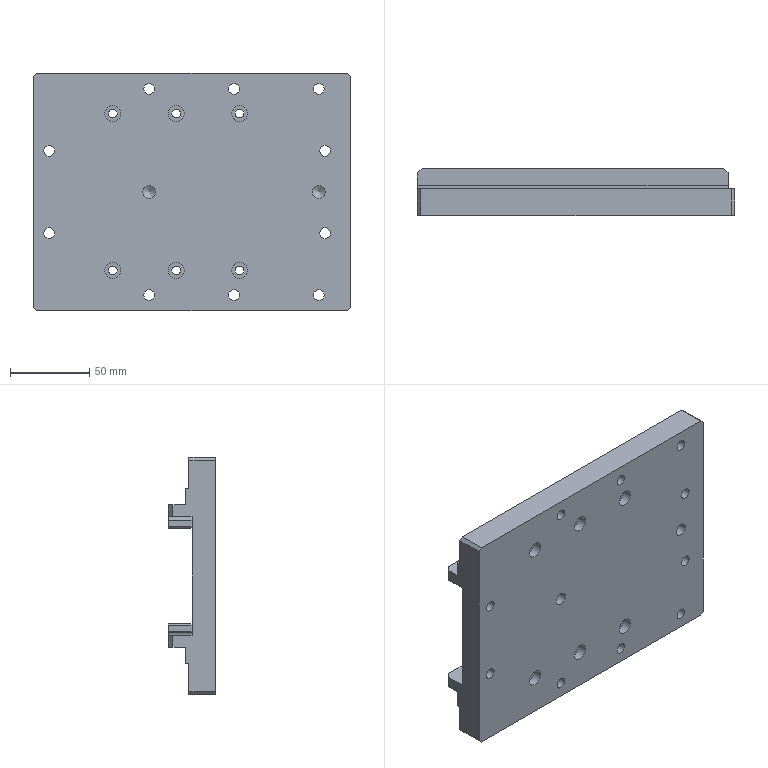CAM job | NX | 3+2 milling, drilling | part box 200 x 30 x 150 mm | stock box 205 x 35 x 155 mm
Tools:
number,name,description,diameter,corner_radius,flute_length,length,flutes
6,D6,平底铣刀-粗,6.0,0.0,25.0,75.0,2
9,D10,平底铣刀-粗,10.0,0.0,35.0,75.0,2
17,D3-J,平底铣刀-精,3.0,0.0,50.0,75.0,2
7,D6-J,平底铣刀-精,6.0,0.0,25.0,75.0,2
10,D10-J,平底铣刀-精,10.0,0.0,35.0,75.0,2
1,D80R0.8飞刀,圆鼻刀-粗,80.0,0.8,50.0,75.0,2
2,D6倒角刀,倒角刀,6.0,0.0,3.0,25.0,2
18,D10倒角刀,倒角刀,10.0,0.0,5.0,75.0,2
19,M8X1.25,丝锥,6.8,0.0,35.0,50.0,2
17,ZT5.5,钻头,5.5,0.0,35.0,50.0,2
16,ZT6.8,钻头,6.8,0.0,35.0,50.0,2
18,ZT7.8,钻头,7.8,0.0,35.0,50.0,2
Operations:
program,operation,operation_type,tool,method,geometry_group,spindle_rpm,surface_speed,feed_per_tooth,feed_cut,feed_plunge,cut_length_mm,path_length_mm,cut_time_min,machine_time_min
B,面铣自动飞面开粗_COPY,FaceMilling,D80R0.8飞刀,分层开粗-切深K-步距G,W-B,4500.0,890.615,0.3333,3000.0,100.0,11397.855,12561.477,3.799,3.916
B,面铣自动飞面精光_COPY,FaceMilling,D80R0.8飞刀,侧刃精光-切深K-步距G,W-B,4500.0,890.615,0.1111,1000.0,100.0,1286.0,1322.0,1.286,1.29
B,型腔铣开粗-中_COPY,CavityMilling,D10,分层开粗-切深K-步距G,W-B,8000.0,251.327,0.3125,5000.0,100.0,106396.675,107852.804,21.279,21.465
B,等高光顺清角D3参考8_COPY,ZLevelMilling,D3-J,分层精光-切深K-步距G,W-B,8000.0,75.398,0.125,2000.0,100.0,7778.73,8343.552,3.889,3.946
B,铣倒角_5,PlanarMilling,D6倒角刀,METHOD,W-B,8000.0,150.796,0.0375,600.0,100.0,237.573,1384.69,0.396,0.5107
B,铣倒角_5_COPY,PlanarMilling,D6倒角刀,METHOD,W-B,8000.0,150.796,0.0375,600.0,100.0,92.54,658.113,0.1542,0.2108
B,平面去毛刺6X45L_COPY,SurfaceContour,D6倒角刀,爬面_倒角-切深0-步距G,W-B,6500.0,122.519,0.1154,1500.0,100.0,2368.766,5559.857,1.579,1.898
B,底壁铣精光底面-中_COPY,VolumeBased25DMillingOperation,D10-J,精光步距切深关,W-B,6000.0,188.496,0.125,1500.0,100.0,1262.86,1426.459,0.8419,0.8583
B,底壁铣精光底面-中_COPY_1,VolumeBased25DMillingOperation,D10-J,精光步距切深关,W-B,6000.0,188.496,0.125,1500.0,100.0,2138.543,2335.209,1.426,1.445
B,底壁铣精光底面-中_COPY_2,VolumeBased25DMillingOperation,D10-J,精光步距切深关,W-B,6000.0,188.496,0.125,1500.0,100.0,2272.714,2328.714,1.515,1.521
B,底壁铣精光侧面-中-选底面_COPY,VolumeBased25DMillingOperation,D10-J,侧刃精光-切深K-步距G,W-B,6000.0,188.496,0.0833,1000.0,100.0,483.926,691.304,0.4839,0.5047
B,底壁铣精光侧面-中-选底面_COPY_1,VolumeBased25DMillingOperation,D10-J,侧刃精光-切深K-步距G,W-B,6000.0,188.496,0.0833,1000.0,100.0,919.744,1152.366,0.9197,0.943
B,底壁铣倒角_COPY,VolumeBased25DMillingOperation,D10倒角刀,爬面_倒角-切深0-步距G,W-B,6500.0,163.358,0.1154,1500.0,100.0,88.113,666.568,0.0587,0.1166
B,底壁铣精光侧面-中-选底面_COPY_2,VolumeBased25DMillingOperation,D10-J,侧刃精光-切深K-步距G,W-B,6000.0,188.496,0.0833,1000.0,100.0,428.566,607.544,0.4286,0.4465
A,顶面,FaceMilling,D80R0.8飞刀,侧刃精光-切深K-步距G,W-A,4000.0,1005.31,0.125,1000.0,100.0,1272.0,1308.0,1.272,1.276
A,外形粗_2,VolumeBased25DMillingOperation,D10,METHOD,W-A,8000.0,251.327,0.3125,5000.0,80.0,29095.835,29164.635,5.819,5.826
A,打点-深0.8,Operation,D6倒角刀,NONE,W-A,8000.0,150.796,0.0312,500.0,90.0,32.4,723.342,0.0648,0.1339
A,沉头孔-钻孔0段,Operation,ZT5.5,NONE,W-A,1200.0,20.735,0.0625,150.0,90.0,141.914,587.883,0.9461,0.9907
A,通孔-M8螺纹底孔,Operation,ZT6.8,NONE,W-A,1800.0,38.453,0.0972,350.0,90.0,262.429,1044.451,0.7498,0.828
A,通孔-精孔8.0预钻14.8,Operation,ZT7.8,NONE,W-A,1500.0,36.757,0.0533,160.0,90.0,24.607,197.218,0.1538,0.1711
A,铣孔开粗D6_1,CylinderMilling,D6,NONE,W-A,8000.0,150.796,0.0312,500.0,100.0,392.26,596.26,0.7845,0.8049
A,铣孔开粗D6_2,CylinderMilling,D6,NONE,W-A,8000.0,150.796,0.075,1200.0,100.0,953.398,1481.798,0.7945,0.8473
A,铣孔精光D6_1,CylinderMilling,D6-J,精光步距切深关,W-A,8000.0,150.796,0.0312,500.0,100.0,200.391,731.791,0.4008,0.4539
A,仅选体,SurfaceContour,D6倒角刀,METHOD,W-A,8000.0,150.796,0.1875,3000.0,100.0,712.615,748.417,0.2375,0.2411
A,铣倒角_1,PlanarMilling,D6倒角刀,METHOD,W-A,8000.0,150.796,0.0375,600.0,100.0,244.012,1129.49,0.4067,0.4952
A,铣倒角_2,PlanarMilling,D6倒角刀,METHOD,W-A,8000.0,150.796,0.0375,600.0,100.0,65.178,258.756,0.1086,0.128
A,铣倒角_3,PlanarMilling,D6倒角刀,NONE,W-A,8000.0,150.796,0.05,800.0,100.0,241.506,725.905,0.3019,0.3503
A,通孔-攻牙M8,Operation,M8X1.25,METHOD,W-A,500.0,10.681,0.0013,1.25,90.0,212.0,943.593,169.6,169.673
A,铣孔精光D6-J_1,CylinderMilling,D6-J,精光步距切深关,W-A,8000.0,150.796,0.0187,300.0,100.0,140.893,344.892,0.4696,0.49
A,外形半精_2,VolumeBased25DMillingOperation,D10-J,METHOD,W-A,8000.0,251.327,0.0625,1000.0,100.0,1463.376,1634.922,1.463,1.48